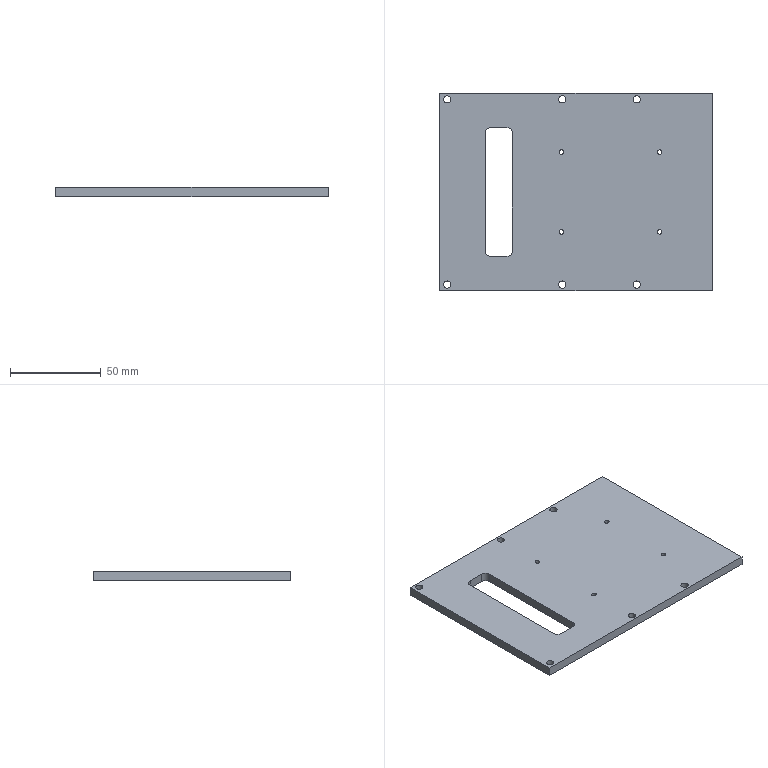NC program | NX | posted with a generic post | part box 150 x 108.5 x 5 mm
Whole program:
N10 G17 G21 G94 G90
(DRILLING , TOOL : D6A45)
N12 T07 M6
N14 G54
N16 G17 G0 G90 X51. Y71. S3500 M3
N18 G43 Z30. H7
N20 G94 G81 G98 Z-2.15 F250. R3.
N22 X22. Y8.
N24 X51. Y7.5
N26 Y-33.5
N28 X22. Y-46.
N30 X-22.
N32 X-51. Y-33.5
N34 Y7.5
N36 X-22. Y8.
N38 X-51. Y71.
N40 G80
N42 G0 X-51. Y71. Z30.
N44 M5
(DRILLING_COPY_COPY_COPY , TOOL : 2.5ZT)
N46 T12 M6
N48 G54
N50 G17 G0 G90 X22. Y8. S2000 M3
N52 G43 Z30. H12
N54 G94 G83 G98 Z-7.251 F120. Q2. R3.
N56 X-22.
N58 Y-46.
N60 X22.
N62 G80
N64 G0 X22. Y-46. Z30.
N66 M5
(DRILLING_COPY_COPY_COPY_COPY , TOOL : 4.0ZT)
N68 T14 M6
N70 G54
N72 G17 G0 G90 X51. Y71. S2000 M3
N74 G43 Z30. H14
N76 G94 G83 G98 Z-7.702 F120. Q2. R3.
N78 Y7.5
N80 Y-33.5
N82 X-51.
N84 Y7.5
N86 Y71.
N88 G80
N90 G0 X-51. Y71. Z30.
N92 M5
(ZLEVEL_PROFILE_2 , TOOL : D10)
N94 T10 M6
N96 G54
N98 G17 G0 G90 X17.697 Y40.15 S9500 M3
N100 G43 Z30. H10
N102 Z1.5
N104 G94 G1 X30.35 Z0.837 F1000.
N106 Y44.85 Z0.591
N108 X0. Z-1.
N110 X-30.35 F2000.
N112 Y40.15
N114 X30.35
N116 Y44.85
N118 X0.
N120 X-30.35 Z-1.53
N122 Y40.15 Z-1.612
N124 X-8.11 Z-2.
N126 X30.35
N128 Y44.85
N130 X0.
N132 X-30.35 Z-2.53
N134 Y40.15 Z-2.612
N136 X-8.11 Z-3.
N138 X30.35
N140 Y44.85
N142 X0.
N144 X-30.35 Z-3.53
N146 Y40.15 Z-3.612
N148 X-8.11 Z-4.
N150 X30.35
N152 Y44.85
N154 X0.
N156 X-30.35 Z-4.53
N158 Y40.15 Z-4.612
N160 X-8.11 Z-5.
N162 X30.35
N164 Y44.85
N166 X-30.35
N168 Y40.15
N170 X-8.11
N172 G3 X-7.244 Y40.65 R1.
N174 G1 X-6.955 Y41.15
N176 Z0.
N178 G0 Z30.
N180 M5
(ZLEVEL_PROFILE_COPY_1 , TOOL : D6)
N182 T06 M6
N184 G54
N186 G17 G0 G90 X-31.9 Y40.909 S9500 M3
N188 G43 Z30. H6
N190 Z-0.5
N192 G94 G1 X-32.2 Y40.736 F1600.
N194 G3 X-32.5 Y40.216 R0.6
N196 G1 Y38.007
N198 X-32.462 Y38.
N200 X-30.284
N202 G3 X-29.764 Y38.3 R0.6
N204 G1 X-29.591 Y38.6
N206 G0 X-31.9 Y40.909 Z-1.
N208 G1 X-32.2 Y40.736
N210 G3 X-32.5 Y40.216 R0.6
N212 G1 Y38.007
N214 X-32.462 Y38.
N216 X-30.284
N218 G3 X-29.764 Y38.3 R0.6
N220 G1 X-29.591 Y38.6
N222 G0 X-31.9 Y40.909 Z-1.5
N224 G1 X-32.2 Y40.736
N226 G3 X-32.5 Y40.216 R0.6
N228 G1 Y38.007
N230 X-32.461 Y38.
N232 X-30.284
N234 G3 X-29.764 Y38.3 R0.6
N236 G1 X-29.591 Y38.6
N238 G0 X-31.9 Y40.909 Z-2.
N240 G1 X-32.2 Y40.736
N242 G3 X-32.5 Y40.216 R0.6
N244 G1 Y38.007
N246 X-32.461 Y38.
N248 X-30.284
N250 G3 X-29.764 Y38.3 R0.6
N252 G1 X-29.591 Y38.6
N254 G0 X-31.9 Y40.909 Z-2.5
N256 G1 X-32.2 Y40.736
N258 G3 X-32.5 Y40.216 R0.6
N260 G1 Y38.008
N262 X-32.461 Y38.
N264 X-30.284
N266 G3 X-29.764 Y38.3 R0.6
N268 G1 X-29.591 Y38.6
N270 G0 X-31.9 Y40.909 Z-3.
N272 G1 X-32.2 Y40.736
N274 G3 X-32.5 Y40.216 R0.6
N276 G1 Y38.008
N278 X-32.461 Y38.
N280 X-30.284
N282 G3 X-29.764 Y38.3 R0.6
N284 G1 X-29.591 Y38.6
N286 G0 X-31.9 Y40.909 Z-3.5
N288 G1 X-32.2 Y40.736
N290 G3 X-32.5 Y40.216 R0.6
N292 G1 Y38.008
N294 X-32.461 Y38.
N296 X-30.284
N298 G3 X-29.764 Y38.3 R0.6
N300 G1 X-29.591 Y38.6
N302 G0 X-31.9 Y40.909 Z-4.
N304 G1 X-32.2 Y40.736
N306 G3 X-32.5 Y40.216 R0.6
N308 G1 Y38.008
N310 X-32.461 Y38.
N312 X-30.284
N314 G3 X-29.764 Y38.3 R0.6
N316 G1 X-29.591 Y38.6
N318 G0 X-31.9 Y40.909 Z-4.5
N320 G1 X-32.2 Y40.736
N322 G3 X-32.5 Y40.216 R0.6
N324 G1 Y38.008
N326 X-32.461 Y38.
N328 X-30.284
N330 G3 X-29.764 Y38.3 R0.6
N332 G1 X-29.591 Y38.6
N334 G0 X-31.9 Y40.909 Z-5.
N336 G1 X-32.2 Y40.736
N338 G3 X-32.5 Y40.216 R0.6
N340 G1 Y38.008
N342 X-32.461 Y38.
N344 X-30.284
N346 G3 X-29.764 Y38.3 R0.6
N348 G1 X-29.591 Y38.6
N350 G0 Z30.
N352 X29.593
N354 Z-0.5
N356 G1 X29.766 Y38.3
N358 G3 X30.286 Y38. R0.6
N360 G1 X32.494
N362 X32.5 Y38.041
N364 Y40.199
N366 G3 X32.2 Y40.719 R0.6
N368 G1 X31.9 Y40.892
N370 G0 X29.593 Y38.6 Z-1.
N372 G1 X29.766 Y38.3
N374 G3 X30.286 Y38. R0.6
N376 G1 X32.494
N378 X32.5 Y38.041
N380 Y40.199
N382 G3 X32.2 Y40.719 R0.6
N384 G1 X31.9 Y40.892
N386 G0 X29.593 Y38.6 Z-1.5
N388 G1 X29.766 Y38.3
N390 G3 X30.286 Y38. R0.6
N392 G1 X32.494
N394 X32.5 Y38.041
N396 Y40.199
N398 G3 X32.2 Y40.719 R0.6
N400 G1 X31.9 Y40.892
N402 G0 X29.593 Y38.6 Z-2.
N404 G1 X29.766 Y38.3
N406 G3 X30.286 Y38. R0.6
N408 G1 X32.494
N410 X32.5 Y38.041
N412 Y40.2
N414 G3 X32.2 Y40.719 R0.6
N416 G1 X31.9 Y40.892
N418 G0 X29.593 Y38.6 Z-2.5
N420 G1 X29.766 Y38.3
N422 G3 X30.286 Y38. R0.6
N424 G1 X32.494
N426 X32.5 Y38.041
N428 Y40.2
N430 G3 X32.2 Y40.719 R0.6
N432 G1 X31.9 Y40.892
N434 G0 X29.593 Y38.6 Z-3.
N436 G1 X29.766 Y38.3
N438 G3 X30.286 Y38. R0.6
N440 G1 X32.494
N442 X32.5 Y38.041
N444 Y40.2
N446 G3 X32.2 Y40.719 R0.6
N448 G1 X31.9 Y40.892
N450 G0 X29.593 Y38.6 Z-3.5
N452 G1 X29.766 Y38.3
N454 G3 X30.286 Y38. R0.6
N456 G1 X32.494
N458 X32.5 Y38.041
N460 Y40.2
N462 G3 X32.2 Y40.719 R0.6
N464 G1 X31.9 Y40.892
N466 G0 X29.593 Y38.6 Z-4.
N468 G1 X29.766 Y38.3
N470 G3 X30.286 Y38. R0.6
N472 G1 X32.494
N474 X32.5 Y38.041
N476 Y40.2
N478 G3 X32.2 Y40.719 R0.6
N480 G1 X31.9 Y40.893
N482 G0 X29.593 Y38.6 Z-4.5
N484 G1 X29.766 Y38.3
N486 G3 X30.286 Y38. R0.6
N488 G1 X32.494
N490 X32.5 Y38.041
N492 Y40.2
N494 G3 X32.2 Y40.719 R0.6
N496 G1 X31.9 Y40.893
N498 G0 X29.593 Y38.6 Z-5.
N500 G1 X29.766 Y38.3
N502 G3 X30.286 Y38. R0.6
N504 G1 X32.494
N506 X32.5 Y38.041
N508 Y40.2
N510 G3 X32.2 Y40.719 R0.6
N512 G1 X31.9 Y40.893
N514 G0 Z30.
N516 Y44.108
N518 Z-0.5
N520 G1 X32.2 Y44.281
N522 G3 X32.5 Y44.801 R0.6
N524 G1 Y46.959
N526 X32.494 Y47.
N528 X30.286
N530 G3 X29.766 Y46.7 R0.6
N532 G1 X29.593 Y46.4
N534 G0 X31.9 Y44.108 Z-1.
N536 G1 X32.2 Y44.281
N538 G3 X32.5 Y44.801 R0.6
N540 G1 Y46.959
N542 X32.494 Y47.
N544 X30.286
N546 G3 X29.766 Y46.7 R0.6
N548 G1 X29.593 Y46.4
N550 G0 X31.9 Y44.108 Z-1.5
N552 G1 X32.2 Y44.281
N554 G3 X32.5 Y44.801 R0.6
N556 G1 Y46.959
N558 X32.494 Y47.
N560 X30.286
N562 G3 X29.766 Y46.7 R0.6
N564 G1 X29.593 Y46.4
N566 G0 X31.9 Y44.108 Z-2.
N568 G1 X32.2 Y44.281
N570 G3 X32.5 Y44.801 R0.6
N572 G1 Y46.959
N574 X32.494 Y47.
N576 X30.286
N578 G3 X29.766 Y46.7 R0.6
N580 G1 X29.593 Y46.4
N582 G0 X31.9 Y44.108 Z-2.5
N584 G1 X32.2 Y44.281
N586 G3 X32.5 Y44.8 R0.6
N588 G1 Y46.959
N590 X32.494 Y47.
N592 X30.286
N594 G3 X29.766 Y46.7 R0.6
N596 G1 X29.593 Y46.4
N598 G0 X31.9 Y44.108 Z-3.
N600 G1 X32.2 Y44.281
N602 G3 X32.5 Y44.8 R0.6
N604 G1 Y46.959
N606 X32.494 Y47.
N608 X30.286
N610 G3 X29.766 Y46.7 R0.6
N612 G1 X29.593 Y46.4
N614 G0 X31.9 Y44.108 Z-3.5
N616 G1 X32.2 Y44.281
N618 G3 X32.5 Y44.8 R0.6
N620 G1 Y46.959
N622 X32.494 Y47.
N624 X30.286
N626 G3 X29.766 Y46.7 R0.6
N628 G1 X29.593 Y46.4
N630 G0 X31.9 Y44.107 Z-4.
N632 G1 X32.2 Y44.281
N634 G3 X32.5 Y44.8 R0.6
N636 G1 Y46.959
N638 X32.494 Y47.
N640 X30.286
N642 G3 X29.766 Y46.7 R0.6
N644 G1 X29.593 Y46.4
N646 G0 X31.9 Y44.107 Z-4.5
N648 G1 X32.2 Y44.281
N650 G3 X32.5 Y44.8 R0.6
N652 G1 Y46.959
N654 X32.494 Y47.
N656 X30.286
N658 G3 X29.766 Y46.7 R0.6
N660 G1 X29.593 Y46.4
N662 G0 X31.9 Y44.107 Z-5.
N664 G1 X32.2 Y44.281
N666 G3 X32.5 Y44.8 R0.6
N668 G1 Y46.959
N670 X32.494 Y47.
N672 X30.286
N674 G3 X29.766 Y46.7 R0.6
N676 G1 X29.593 Y46.4
N678 G0 Z30.
N680 X-29.591
N682 Z-0.5
N684 G1 X-29.764 Y46.7
N686 G3 X-30.284 Y47. R0.6
N688 G1 X-32.462
N690 X-32.5 Y46.993
N692 Y44.784
N694 G3 X-32.2 Y44.264 R0.6
N696 G1 X-31.9 Y44.091
N698 G0 X-29.591 Y46.4 Z-1.
N700 G1 X-29.764 Y46.7
N702 G3 X-30.284 Y47. R0.6
N704 G1 X-32.462
N706 X-32.5 Y46.993
N708 Y44.784
N710 G3 X-32.2 Y44.264 R0.6
N712 G1 X-31.9 Y44.091
N714 G0 X-29.591 Y46.4 Z-1.5
N716 G1 X-29.764 Y46.7
N718 G3 X-30.284 Y47. R0.6
N720 G1 X-32.461
N722 X-32.5 Y46.993
N724 Y44.784
N726 G3 X-32.2 Y44.264 R0.6
N728 G1 X-31.9 Y44.091
N730 G0 X-29.591 Y46.4 Z-2.
N732 G1 X-29.764 Y46.7
N734 G3 X-30.284 Y47. R0.6
N736 G1 X-32.461
N738 X-32.5 Y46.993
N740 Y44.784
N742 G3 X-32.2 Y44.264 R0.6
N744 G1 X-31.9 Y44.091
N746 G0 X-29.591 Y46.4 Z-2.5
N748 G1 X-29.764 Y46.7
N750 G3 X-30.284 Y47. R0.6
N752 G1 X-32.461
N754 X-32.5 Y46.992
N756 Y44.784
N758 G3 X-32.2 Y44.264 R0.6
N760 G1 X-31.9 Y44.091
N762 G0 X-29.591 Y46.4 Z-3.
N764 G1 X-29.764 Y46.7
N766 G3 X-30.284 Y47. R0.6
N768 G1 X-32.461
N770 X-32.5 Y46.992
N772 Y44.784
N774 G3 X-32.2 Y44.264 R0.6
N776 G1 X-31.9 Y44.091
N778 G0 X-29.591 Y46.4 Z-3.5
N780 G1 X-29.764 Y46.7
N782 G3 X-30.284 Y47. R0.6
N784 G1 X-32.461
N786 X-32.5 Y46.992
N788 Y44.784
N790 G3 X-32.2 Y44.264 R0.6
N792 G1 X-31.9 Y44.091
N794 G0 X-29.591 Y46.4 Z-4.
N796 G1 X-29.764 Y46.7
N798 G3 X-30.284 Y47. R0.6
N800 G1 X-32.461
N802 X-32.5 Y46.992
N804 Y44.784
N806 G3 X-32.2 Y44.264 R0.6
N808 G1 X-31.9 Y44.091
N810 G0 X-29.591 Y46.4 Z-4.5
N812 G1 X-29.764 Y46.7
N814 G3 X-30.284 Y47. R0.6
N816 G1 X-32.461
N818 X-32.5 Y46.992
N820 Y44.784
N822 G3 X-32.2 Y44.264 R0.6
N824 G1 X-31.9 Y44.091
N826 G0 X-29.591 Y46.4 Z-5.
N828 G1 X-29.764 Y46.7
N830 G3 X-30.284 Y47. R0.6
N832 G1 X-32.461
N834 X-32.5 Y46.992
N836 Y44.784
N838 G3 X-32.2 Y44.264 R0.6
N840 G1 X-31.9 Y44.091
N842 G0 Z30.
(ZLEVEL_PROFILE_1 , TOOL : D6)
N844 X31.3 Y45.784
N846 Z-3.5
N848 G1 Z-5. F1000.
N850 X31.494 Y45.818
N852 G3 X32.486 Y47. R1.2
N854 G1 X-32.444
N856 X-32.5 Y46.992
N858 Y38.008
N860 X-32.444 Y38.
N862 X32.486
N864 X32.489 Y38.003
N866 X32.5 Y38.06
N868 Y46.94
N870 X32.489 Y46.997
N872 X32.486 Y47.
N874 G3 X31.304 Y46.008 R1.2
N876 G1 X31.267 Y45.8
N878 Z-3.5
N880 G0 Z30.
N882 M5
(ZLEVEL_PROFILE_1_COPY_1_COPY_COPY_COPY_1 , TOOL : D6A45)
N884 T07 M6
N886 G54
N888 G17 G0 G90 X52.041 Y71. S9500 M3
N890 G43 Z30. H7
N892 Z1.
N894 G94 G1 Z-1. F1000.
N896 G3 X51. Y72.041 R1.041
N898 X52.041 Y71. R-1.041
N900 X51.741 Y71.52 R0.6
N902 G1 Z0.
N904 G0 Z30.
N906 X22. Y-46.291
N908 Z1.
N910 G1 Z-1.
N912 G3 X22.291 Y-46. R0.291
N914 X22. Y-46.291 R-0.291
N916 X22.26 Y-46.141 R0.3
N918 G1 Z0.
N920 G0 Z30.
N922 X22.291 Y8.
N924 Z1.
N926 G1 Z-1.
N928 G3 X22. Y8.291 R0.291
N930 X22.291 Y8. R-0.291
N932 X22.141 Y8.26 R0.3
N934 G1 Z0.
N936 G0 Z30.
N938 X-22. Y-46.291
N940 Z1.
N942 G1 Z-1.
N944 G3 X-21.709 Y-46. R0.291
N946 X-22. Y-46.291 R-0.291
N948 X-21.74 Y-46.141 R0.3
N950 G1 Z0.
N952 G0 Z30.
N954 X-22.291 Y8.
N956 Z1.
N958 G1 Z-1.
N960 G3 X-22. Y7.709 R0.291
N962 X-22.291 Y8. R-0.291
N964 X-22.141 Y7.74 R0.3
N966 G1 Z0.
N968 G0 Z30.
N970 X52.041 Y-33.5
N972 Z1.
N974 G1 Z-1.
N976 G3 X51. Y-32.459 R1.041
N978 X52.041 Y-33.5 R-1.041
N980 X51.741 Y-32.98 R0.6
N982 G1 Z0.
N984 G0 Z30.
N986 X32.741 Y47.806
N988 Z0.
N990 G1 Z-1.
N992 X33.02 Y48.741
N994 G3 X32.5 Y49.041 R0.6
N996 G1 X-32.5
N998 G3 X-34.541 Y47. R2.041
N1000 G1 Y38.
N1002 G3 X-32.5 Y35.959 R2.041
N1004 G1 X32.5
N1006 G3 X34.541 Y38. R2.041
N1008 G1 Y47.
N1010 G3 X32.5 Y49.041 R2.041
N1012 X31.98 Y48.741 R0.6
N1014 G1 X31.461 Y47.841
N1016 Z0.
N1018 G0 Z30.
N1020 X-52.041 Y-33.5
N1022 Z1.
N1024 G1 Z-1.
N1026 G3 X-51. Y-34.541 R1.041
N1028 X-52.041 Y-33.5 R-1.041
N1030 X-51.741 Y-34.02 R0.6
N1032 G1 Z0.
N1034 G0 Z30.
N1036 X-52.041 Y7.5
N1038 Z1.
N1040 G1 Z-1.
N1042 G3 X-51. Y6.459 R1.041
N1044 X-52.041 Y7.5 R-1.041
N1046 X-51.741 Y6.98 R0.6
N1048 G1 Z0.
N1050 G0 Z30.
N1052 X-52.041 Y71.
N1054 Z1.
N1056 G1 Z-1.
N1058 G3 X-51. Y69.959 R1.041
N1060 X-52.041 Y71. R-1.041
N1062 X-51.741 Y70.48 R0.6
N1064 G1 Z0.
N1066 G0 Z30.
N1068 X52.041 Y7.5
N1070 Z1.
N1072 G1 Z-1.
N1074 G3 X51. Y8.541 R1.041
N1076 X52.041 Y7.5 R-1.041
N1078 X51.741 Y8.02 R0.6
N1080 G1 Z0.
N1082 G0 Z30.
N1084 M5
N1086 M2